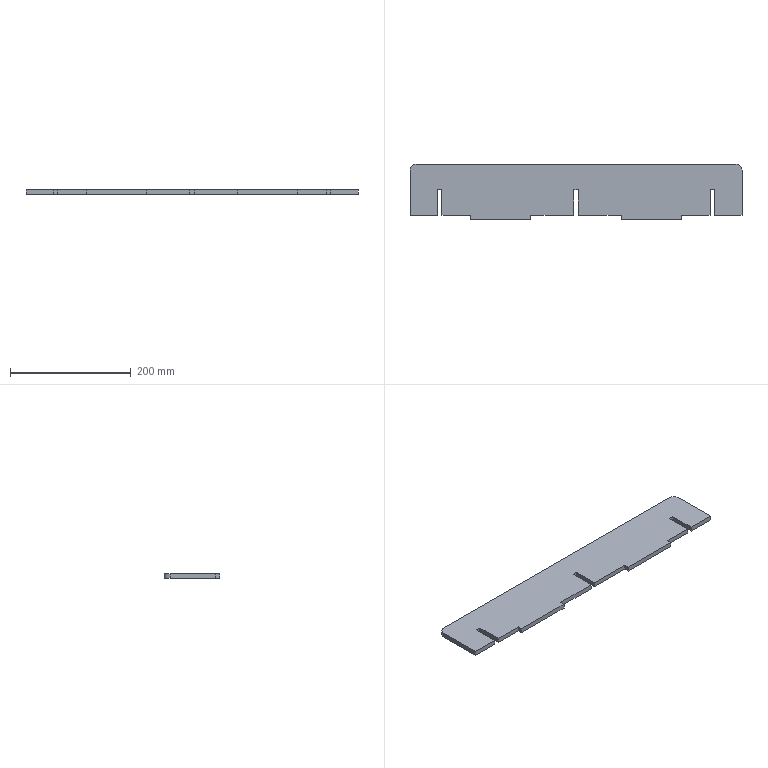Part | SolidWorks | features FlatPattern 1, SMBaseFlange 1, SheetMetal 1 | 1 solid | 28 faces | box 550 x 92.5 x 8 mm | volume 377497 mm3 | plane 26 | cylinder 2 | commonest cylinder face diameters 20 x2
STEP:
#1=CARTESIAN_POINT('',(-156.899,-982.506,0.));
#2=VERTEX_POINT('',#1);
#3=CARTESIAN_POINT('',(-111.899,-982.506,0.));
#4=VERTEX_POINT('',#3);
#5=CARTESIAN_POINT('',(-111.899,-982.506,0.));
#6=DIRECTION('',(1.,0.,0.));
#7=VECTOR('',#6,1000.);
#8=LINE('',#5,#7);
#9=EDGE_CURVE('',#2,#4,#8,.T.);
#10=ORIENTED_EDGE('',*,*,#9,.F.);
#11=CARTESIAN_POINT('',(-156.899,-982.506,-8.));
#12=VERTEX_POINT('',#11);
#13=CARTESIAN_POINT('',(-156.899,-982.506,-8.));
#14=DIRECTION('',(0.,0.,1.));
#15=VECTOR('',#14,1000.);
#16=LINE('',#13,#15);
#17=EDGE_CURVE('',#12,#2,#16,.T.);
#18=ORIENTED_EDGE('',*,*,#17,.F.);
#19=CARTESIAN_POINT('',(-111.899,-982.506,-8.));
#20=VERTEX_POINT('',#19);
#21=CARTESIAN_POINT('',(-111.899,-982.506,-8.));
#22=DIRECTION('',(1.,0.,0.));
#23=VECTOR('',#22,1000.);
#24=LINE('',#21,#23);
#25=EDGE_CURVE('',#12,#20,#24,.T.);
#26=ORIENTED_EDGE('',*,*,#25,.T.);
#27=CARTESIAN_POINT('',(-111.899,-982.506,-8.));
#28=DIRECTION('',(0.,0.,1.));
#29=VECTOR('',#28,1000.);
#30=LINE('',#27,#29);
#31=EDGE_CURVE('',#20,#4,#30,.T.);
#32=ORIENTED_EDGE('',*,*,#31,.T.);
#33=EDGE_LOOP('',(#10,#18,#26,#32));
#34=FACE_OUTER_BOUND('',#33,.T.);
#35=CARTESIAN_POINT('',(-111.899,-982.506,-8.));
#36=DIRECTION('',(0.,-1.,0.));
#37=DIRECTION('',(0.,0.,-1.));
#38=AXIS2_PLACEMENT_3D('',#35,#36,#37);
#39=PLANE('',#38);
#40=ADVANCED_FACE('',(#34),#39,.T.);
#41=CARTESIAN_POINT('',(-156.899,-907.506,0.));
#42=VERTEX_POINT('',#41);
#43=CARTESIAN_POINT('',(-156.899,-982.506,0.));
#44=DIRECTION('',(0.,-1.,0.));
#45=VECTOR('',#44,1000.);
#46=LINE('',#43,#45);
#47=EDGE_CURVE('',#42,#2,#46,.T.);
#48=ORIENTED_EDGE('',*,*,#47,.F.);
#49=CARTESIAN_POINT('',(-156.899,-907.506,-8.));
#50=VERTEX_POINT('',#49);
#51=CARTESIAN_POINT('',(-156.899,-907.506,-8.));
#52=DIRECTION('',(0.,0.,1.));
#53=VECTOR('',#52,1000.);
#54=LINE('',#51,#53);
#55=EDGE_CURVE('',#50,#42,#54,.T.);
#56=ORIENTED_EDGE('',*,*,#55,.F.);
#57=CARTESIAN_POINT('',(-156.899,-982.506,-8.));
#58=DIRECTION('',(0.,-1.,0.));
#59=VECTOR('',#58,1000.);
#60=LINE('',#57,#59);
#61=EDGE_CURVE('',#50,#12,#60,.T.);
#62=ORIENTED_EDGE('',*,*,#61,.T.);
#63=ORIENTED_EDGE('',*,*,#17,.T.);
#64=EDGE_LOOP('',(#48,#56,#62,#63));
#65=FACE_OUTER_BOUND('',#64,.T.);
#66=CARTESIAN_POINT('',(-156.899,-982.506,-8.));
#67=DIRECTION('',(-1.,0.,0.));
#68=DIRECTION('',(0.,0.,1.));
#69=AXIS2_PLACEMENT_3D('',#66,#67,#68);
#70=PLANE('',#69);
#71=ADVANCED_FACE('',(#65),#70,.T.);
#72=CARTESIAN_POINT('',(-146.899,-897.506,0.));
#73=VERTEX_POINT('',#72);
#74=CARTESIAN_POINT('',(-146.899,-907.506,0.));
#75=DIRECTION('',(0.,0.,1.));
#76=DIRECTION('',(-1.,0.,0.));
#77=AXIS2_PLACEMENT_3D('',#74,#75,#76);
#78=CIRCLE('',#77,10.);
#79=EDGE_CURVE('',#73,#42,#78,.T.);
#80=ORIENTED_EDGE('',*,*,#79,.F.);
#81=CARTESIAN_POINT('',(-146.899,-897.506,-8.));
#82=VERTEX_POINT('',#81);
#83=CARTESIAN_POINT('',(-146.899,-897.506,-8.));
#84=DIRECTION('',(0.,0.,1.));
#85=VECTOR('',#84,1000.);
#86=LINE('',#83,#85);
#87=EDGE_CURVE('',#82,#73,#86,.T.);
#88=ORIENTED_EDGE('',*,*,#87,.F.);
#89=CARTESIAN_POINT('',(-146.899,-907.506,-8.));
#90=DIRECTION('',(0.,0.,1.));
#91=DIRECTION('',(-1.,0.,0.));
#92=AXIS2_PLACEMENT_3D('',#89,#90,#91);
#93=CIRCLE('',#92,10.);
#94=EDGE_CURVE('',#82,#50,#93,.T.);
#95=ORIENTED_EDGE('',*,*,#94,.T.);
#96=ORIENTED_EDGE('',*,*,#55,.T.);
#97=EDGE_LOOP('',(#80,#88,#95,#96));
#98=FACE_OUTER_BOUND('',#97,.T.);
#99=CARTESIAN_POINT('',(-146.899,-907.506,-8.));
#100=DIRECTION('',(0.,0.,1.));
#101=DIRECTION('',(1.,0.,0.));
#102=AXIS2_PLACEMENT_3D('',#99,#100,#101);
#103=CYLINDRICAL_SURFACE('',#102,10.);
#104=ADVANCED_FACE('',(#98),#103,.T.);
#105=CARTESIAN_POINT('',(383.101,-897.506,0.));
#106=VERTEX_POINT('',#105);
#107=CARTESIAN_POINT('',(-146.899,-897.506,0.));
#108=DIRECTION('',(-1.,0.,0.));
#109=VECTOR('',#108,1000.);
#110=LINE('',#107,#109);
#111=EDGE_CURVE('',#106,#73,#110,.T.);
#112=ORIENTED_EDGE('',*,*,#111,.F.);
#113=CARTESIAN_POINT('',(383.101,-897.506,-8.));
#114=VERTEX_POINT('',#113);
#115=CARTESIAN_POINT('',(383.101,-897.506,-8.));
#116=DIRECTION('',(0.,0.,1.));
#117=VECTOR('',#116,1000.);
#118=LINE('',#115,#117);
#119=EDGE_CURVE('',#114,#106,#118,.T.);
#120=ORIENTED_EDGE('',*,*,#119,.F.);
#121=CARTESIAN_POINT('',(-146.899,-897.506,-8.));
#122=DIRECTION('',(-1.,0.,0.));
#123=VECTOR('',#122,1000.);
#124=LINE('',#121,#123);
#125=EDGE_CURVE('',#114,#82,#124,.T.);
#126=ORIENTED_EDGE('',*,*,#125,.T.);
#127=ORIENTED_EDGE('',*,*,#87,.T.);
#128=EDGE_LOOP('',(#112,#120,#126,#127));
#129=FACE_OUTER_BOUND('',#128,.T.);
#130=CARTESIAN_POINT('',(-146.899,-897.506,-8.));
#131=DIRECTION('',(0.,1.,0.));
#132=DIRECTION('',(0.,0.,1.));
#133=AXIS2_PLACEMENT_3D('',#130,#131,#132);
#134=PLANE('',#133);
#135=ADVANCED_FACE('',(#129),#134,.T.);
#136=CARTESIAN_POINT('',(393.101,-907.506,0.));
#137=VERTEX_POINT('',#136);
#138=CARTESIAN_POINT('',(383.101,-907.506,0.));
#139=DIRECTION('',(0.,0.,1.));
#140=DIRECTION('',(-1.,0.,0.));
#141=AXIS2_PLACEMENT_3D('',#138,#139,#140);
#142=CIRCLE('',#141,10.);
#143=EDGE_CURVE('',#137,#106,#142,.T.);
#144=ORIENTED_EDGE('',*,*,#143,.F.);
#145=CARTESIAN_POINT('',(393.101,-907.506,-8.));
#146=VERTEX_POINT('',#145);
#147=CARTESIAN_POINT('',(393.101,-907.506,-8.));
#148=DIRECTION('',(0.,0.,1.));
#149=VECTOR('',#148,1000.);
#150=LINE('',#147,#149);
#151=EDGE_CURVE('',#146,#137,#150,.T.);
#152=ORIENTED_EDGE('',*,*,#151,.F.);
#153=CARTESIAN_POINT('',(383.101,-907.506,-8.));
#154=DIRECTION('',(0.,0.,1.));
#155=DIRECTION('',(-1.,0.,0.));
#156=AXIS2_PLACEMENT_3D('',#153,#154,#155);
#157=CIRCLE('',#156,10.);
#158=EDGE_CURVE('',#146,#114,#157,.T.);
#159=ORIENTED_EDGE('',*,*,#158,.T.);
#160=ORIENTED_EDGE('',*,*,#119,.T.);
#161=EDGE_LOOP('',(#144,#152,#159,#160));
#162=FACE_OUTER_BOUND('',#161,.T.);
#163=CARTESIAN_POINT('',(383.101,-907.506,-8.));
#164=DIRECTION('',(0.,0.,1.));
#165=DIRECTION('',(1.,0.,0.));
#166=AXIS2_PLACEMENT_3D('',#163,#164,#165);
#167=CYLINDRICAL_SURFACE('',#166,10.);
#168=ADVANCED_FACE('',(#162),#167,.T.);
#169=CARTESIAN_POINT('',(393.101,-982.506,0.));
#170=VERTEX_POINT('',#169);
#171=CARTESIAN_POINT('',(393.101,-907.506,0.));
#172=DIRECTION('',(0.,1.,0.));
#173=VECTOR('',#172,1000.);
#174=LINE('',#171,#173);
#175=EDGE_CURVE('',#170,#137,#174,.T.);
#176=ORIENTED_EDGE('',*,*,#175,.F.);
#177=CARTESIAN_POINT('',(393.101,-982.506,-8.));
#178=VERTEX_POINT('',#177);
#179=CARTESIAN_POINT('',(393.101,-982.506,-8.));
#180=DIRECTION('',(0.,0.,1.));
#181=VECTOR('',#180,1000.);
#182=LINE('',#179,#181);
#183=EDGE_CURVE('',#178,#170,#182,.T.);
#184=ORIENTED_EDGE('',*,*,#183,.F.);
#185=CARTESIAN_POINT('',(393.101,-907.506,-8.));
#186=DIRECTION('',(0.,1.,0.));
#187=VECTOR('',#186,1000.);
#188=LINE('',#185,#187);
#189=EDGE_CURVE('',#178,#146,#188,.T.);
#190=ORIENTED_EDGE('',*,*,#189,.T.);
#191=ORIENTED_EDGE('',*,*,#151,.T.);
#192=EDGE_LOOP('',(#176,#184,#190,#191));
#193=FACE_OUTER_BOUND('',#192,.T.);
#194=CARTESIAN_POINT('',(393.101,-907.506,-8.));
#195=DIRECTION('',(1.,0.,0.));
#196=DIRECTION('',(0.,0.,-1.));
#197=AXIS2_PLACEMENT_3D('',#194,#195,#196);
#198=PLANE('',#197);
#199=ADVANCED_FACE('',(#193),#198,.T.);
#200=CARTESIAN_POINT('',(348.101,-982.506,0.));
#201=VERTEX_POINT('',#200);
#202=CARTESIAN_POINT('',(393.101,-982.506,0.));
#203=DIRECTION('',(1.,0.,0.));
#204=VECTOR('',#203,1000.);
#205=LINE('',#202,#204);
#206=EDGE_CURVE('',#201,#170,#205,.T.);
#207=ORIENTED_EDGE('',*,*,#206,.F.);
#208=CARTESIAN_POINT('',(348.101,-982.506,-8.));
#209=VERTEX_POINT('',#208);
#210=CARTESIAN_POINT('',(348.101,-982.506,-8.));
#211=DIRECTION('',(0.,0.,1.));
#212=VECTOR('',#211,1000.);
#213=LINE('',#210,#212);
#214=EDGE_CURVE('',#209,#201,#213,.T.);
#215=ORIENTED_EDGE('',*,*,#214,.F.);
#216=CARTESIAN_POINT('',(393.101,-982.506,-8.));
#217=DIRECTION('',(1.,0.,0.));
#218=VECTOR('',#217,1000.);
#219=LINE('',#216,#218);
#220=EDGE_CURVE('',#209,#178,#219,.T.);
#221=ORIENTED_EDGE('',*,*,#220,.T.);
#222=ORIENTED_EDGE('',*,*,#183,.T.);
#223=EDGE_LOOP('',(#207,#215,#221,#222));
#224=FACE_OUTER_BOUND('',#223,.T.);
#225=CARTESIAN_POINT('',(393.101,-982.506,-8.));
#226=DIRECTION('',(0.,-1.,0.));
#227=DIRECTION('',(0.,0.,-1.));
#228=AXIS2_PLACEMENT_3D('',#225,#226,#227);
#229=PLANE('',#228);
#230=ADVANCED_FACE('',(#224),#229,.T.);
#231=CARTESIAN_POINT('',(348.101,-940.006,0.));
#232=VERTEX_POINT('',#231);
#233=CARTESIAN_POINT('',(348.101,-982.506,0.));
#234=DIRECTION('',(0.,-1.,0.));
#235=VECTOR('',#234,1000.);
#236=LINE('',#233,#235);
#237=EDGE_CURVE('',#232,#201,#236,.T.);
#238=ORIENTED_EDGE('',*,*,#237,.F.);
#239=CARTESIAN_POINT('',(348.101,-940.006,-8.));
#240=VERTEX_POINT('',#239);
#241=CARTESIAN_POINT('',(348.101,-940.006,-8.));
#242=DIRECTION('',(0.,0.,1.));
#243=VECTOR('',#242,1000.);
#244=LINE('',#241,#243);
#245=EDGE_CURVE('',#240,#232,#244,.T.);
#246=ORIENTED_EDGE('',*,*,#245,.F.);
#247=CARTESIAN_POINT('',(348.101,-982.506,-8.));
#248=DIRECTION('',(0.,-1.,0.));
#249=VECTOR('',#248,1000.);
#250=LINE('',#247,#249);
#251=EDGE_CURVE('',#240,#209,#250,.T.);
#252=ORIENTED_EDGE('',*,*,#251,.T.);
#253=ORIENTED_EDGE('',*,*,#214,.T.);
#254=EDGE_LOOP('',(#238,#246,#252,#253));
#255=FACE_OUTER_BOUND('',#254,.T.);
#256=CARTESIAN_POINT('',(348.101,-982.506,-8.));
#257=DIRECTION('',(-1.,0.,0.));
#258=DIRECTION('',(0.,0.,1.));
#259=AXIS2_PLACEMENT_3D('',#256,#257,#258);
#260=PLANE('',#259);
#261=ADVANCED_FACE('',(#255),#260,.T.);
#262=CARTESIAN_POINT('',(340.101,-940.006,0.));
#263=VERTEX_POINT('',#262);
#264=CARTESIAN_POINT('',(348.101,-940.006,0.));
#265=DIRECTION('',(1.,0.,0.));
#266=VECTOR('',#265,1000.);
#267=LINE('',#264,#266);
#268=EDGE_CURVE('',#263,#232,#267,.T.);
#269=ORIENTED_EDGE('',*,*,#268,.F.);
#270=CARTESIAN_POINT('',(340.101,-940.006,-8.));
#271=VERTEX_POINT('',#270);
#272=CARTESIAN_POINT('',(340.101,-940.006,-8.));
#273=DIRECTION('',(0.,0.,1.));
#274=VECTOR('',#273,1000.);
#275=LINE('',#272,#274);
#276=EDGE_CURVE('',#271,#263,#275,.T.);
#277=ORIENTED_EDGE('',*,*,#276,.F.);
#278=CARTESIAN_POINT('',(348.101,-940.006,-8.));
#279=DIRECTION('',(1.,0.,0.));
#280=VECTOR('',#279,1000.);
#281=LINE('',#278,#280);
#282=EDGE_CURVE('',#271,#240,#281,.T.);
#283=ORIENTED_EDGE('',*,*,#282,.T.);
#284=ORIENTED_EDGE('',*,*,#245,.T.);
#285=EDGE_LOOP('',(#269,#277,#283,#284));
#286=FACE_OUTER_BOUND('',#285,.T.);
#287=CARTESIAN_POINT('',(348.101,-940.006,-8.));
#288=DIRECTION('',(0.,-1.,0.));
#289=DIRECTION('',(0.,0.,-1.));
#290=AXIS2_PLACEMENT_3D('',#287,#288,#289);
#291=PLANE('',#290);
#292=ADVANCED_FACE('',(#286),#291,.T.);
#293=CARTESIAN_POINT('',(340.101,-982.506,0.));
#294=VERTEX_POINT('',#293);
#295=CARTESIAN_POINT('',(340.101,-940.006,0.));
#296=DIRECTION('',(0.,1.,0.));
#297=VECTOR('',#296,1000.);
#298=LINE('',#295,#297);
#299=EDGE_CURVE('',#294,#263,#298,.T.);
#300=ORIENTED_EDGE('',*,*,#299,.F.);
#301=CARTESIAN_POINT('',(340.101,-982.506,-8.));
#302=VERTEX_POINT('',#301);
#303=CARTESIAN_POINT('',(340.101,-982.506,-8.));
#304=DIRECTION('',(0.,0.,1.));
#305=VECTOR('',#304,1000.);
#306=LINE('',#303,#305);
#307=EDGE_CURVE('',#302,#294,#306,.T.);
#308=ORIENTED_EDGE('',*,*,#307,.F.);
#309=CARTESIAN_POINT('',(340.101,-940.006,-8.));
#310=DIRECTION('',(0.,1.,0.));
#311=VECTOR('',#310,1000.);
#312=LINE('',#309,#311);
#313=EDGE_CURVE('',#302,#271,#312,.T.);
#314=ORIENTED_EDGE('',*,*,#313,.T.);
#315=ORIENTED_EDGE('',*,*,#276,.T.);
#316=EDGE_LOOP('',(#300,#308,#314,#315));
#317=FACE_OUTER_BOUND('',#316,.T.);
#318=CARTESIAN_POINT('',(340.101,-940.006,-8.));
#319=DIRECTION('',(1.,0.,0.));
#320=DIRECTION('',(0.,0.,-1.));
#321=AXIS2_PLACEMENT_3D('',#318,#319,#320);
#322=PLANE('',#321);
#323=ADVANCED_FACE('',(#317),#322,.T.);
#324=CARTESIAN_POINT('',(293.101,-982.506,0.));
#325=VERTEX_POINT('',#324);
#326=CARTESIAN_POINT('',(340.101,-982.506,0.));
#327=DIRECTION('',(1.,0.,0.));
#328=VECTOR('',#327,1000.);
#329=LINE('',#326,#328);
#330=EDGE_CURVE('',#325,#294,#329,.T.);
#331=ORIENTED_EDGE('',*,*,#330,.F.);
#332=CARTESIAN_POINT('',(293.101,-982.506,-8.));
#333=VERTEX_POINT('',#332);
#334=CARTESIAN_POINT('',(293.101,-982.506,-8.));
#335=DIRECTION('',(0.,0.,1.));
#336=VECTOR('',#335,1000.);
#337=LINE('',#334,#336);
#338=EDGE_CURVE('',#333,#325,#337,.T.);
#339=ORIENTED_EDGE('',*,*,#338,.F.);
#340=CARTESIAN_POINT('',(340.101,-982.506,-8.));
#341=DIRECTION('',(1.,0.,0.));
#342=VECTOR('',#341,1000.);
#343=LINE('',#340,#342);
#344=EDGE_CURVE('',#333,#302,#343,.T.);
#345=ORIENTED_EDGE('',*,*,#344,.T.);
#346=ORIENTED_EDGE('',*,*,#307,.T.);
#347=EDGE_LOOP('',(#331,#339,#345,#346));
#348=FACE_OUTER_BOUND('',#347,.T.);
#349=CARTESIAN_POINT('',(340.101,-982.506,-8.));
#350=DIRECTION('',(0.,-1.,0.));
#351=DIRECTION('',(1.,0.,0.));
#352=AXIS2_PLACEMENT_3D('',#349,#350,#351);
#353=PLANE('',#352);
#354=ADVANCED_FACE('',(#348),#353,.T.);
#355=CARTESIAN_POINT('',(293.101,-990.006,0.));
#356=VERTEX_POINT('',#355);
#357=CARTESIAN_POINT('',(293.101,-990.006,0.));
#358=DIRECTION('',(0.,1.,0.));
#359=VECTOR('',#358,1000.);
#360=LINE('',#357,#359);
#361=EDGE_CURVE('',#356,#325,#360,.T.);
#362=ORIENTED_EDGE('',*,*,#361,.F.);
#363=CARTESIAN_POINT('',(293.101,-990.006,-8.));
#364=VERTEX_POINT('',#363);
#365=CARTESIAN_POINT('',(293.101,-990.006,-8.));
#366=DIRECTION('',(0.,0.,1.));
#367=VECTOR('',#366,1000.);
#368=LINE('',#365,#367);
#369=EDGE_CURVE('',#364,#356,#368,.T.);
#370=ORIENTED_EDGE('',*,*,#369,.F.);
#371=CARTESIAN_POINT('',(293.101,-990.006,-8.));
#372=DIRECTION('',(0.,1.,0.));
#373=VECTOR('',#372,1000.);
#374=LINE('',#371,#373);
#375=EDGE_CURVE('',#364,#333,#374,.T.);
#376=ORIENTED_EDGE('',*,*,#375,.T.);
#377=ORIENTED_EDGE('',*,*,#338,.T.);
#378=EDGE_LOOP('',(#362,#370,#376,#377));
#379=FACE_OUTER_BOUND('',#378,.T.);
#380=CARTESIAN_POINT('',(293.101,-990.006,-8.));
#381=DIRECTION('',(1.,0.,0.));
#382=DIRECTION('',(0.,0.,-1.));
#383=AXIS2_PLACEMENT_3D('',#380,#381,#382);
#384=PLANE('',#383);
#385=ADVANCED_FACE('',(#379),#384,.T.);
#386=CARTESIAN_POINT('',(193.101,-990.006,0.));
#387=VERTEX_POINT('',#386);
#388=CARTESIAN_POINT('',(193.101,-990.006,0.));
#389=DIRECTION('',(1.,0.,0.));
#390=VECTOR('',#389,1000.);
#391=LINE('',#388,#390);
#392=EDGE_CURVE('',#387,#356,#391,.T.);
#393=ORIENTED_EDGE('',*,*,#392,.F.);
#394=CARTESIAN_POINT('',(193.101,-990.006,-8.));
#395=VERTEX_POINT('',#394);
#396=CARTESIAN_POINT('',(193.101,-990.006,-8.));
#397=DIRECTION('',(0.,0.,1.));
#398=VECTOR('',#397,1000.);
#399=LINE('',#396,#398);
#400=EDGE_CURVE('',#395,#387,#399,.T.);
#401=ORIENTED_EDGE('',*,*,#400,.F.);
#402=CARTESIAN_POINT('',(193.101,-990.006,-8.));
#403=DIRECTION('',(1.,0.,0.));
#404=VECTOR('',#403,1000.);
#405=LINE('',#402,#404);
#406=EDGE_CURVE('',#395,#364,#405,.T.);
#407=ORIENTED_EDGE('',*,*,#406,.T.);
#408=ORIENTED_EDGE('',*,*,#369,.T.);
#409=EDGE_LOOP('',(#393,#401,#407,#408));
#410=FACE_OUTER_BOUND('',#409,.T.);
#411=CARTESIAN_POINT('',(193.101,-990.006,-8.));
#412=DIRECTION('',(0.,-1.,0.));
#413=DIRECTION('',(0.,0.,-1.));
#414=AXIS2_PLACEMENT_3D('',#411,#412,#413);
#415=PLANE('',#414);
#416=ADVANCED_FACE('',(#410),#415,.T.);
#417=CARTESIAN_POINT('',(193.101,-982.506,0.));
#418=VERTEX_POINT('',#417);
#419=CARTESIAN_POINT('',(193.101,-982.506,0.));
#420=DIRECTION('',(0.,-1.,0.));
#421=VECTOR('',#420,1000.);
#422=LINE('',#419,#421);
#423=EDGE_CURVE('',#418,#387,#422,.T.);
#424=ORIENTED_EDGE('',*,*,#423,.F.);
#425=CARTESIAN_POINT('',(193.101,-982.506,-8.));
#426=VERTEX_POINT('',#425);
#427=CARTESIAN_POINT('',(193.101,-982.506,-8.));
#428=DIRECTION('',(0.,0.,1.));
#429=VECTOR('',#428,1000.);
#430=LINE('',#427,#429);
#431=EDGE_CURVE('',#426,#418,#430,.T.);
#432=ORIENTED_EDGE('',*,*,#431,.F.);
#433=CARTESIAN_POINT('',(193.101,-982.506,-8.));
#434=DIRECTION('',(0.,-1.,0.));
#435=VECTOR('',#434,1000.);
#436=LINE('',#433,#435);
#437=EDGE_CURVE('',#426,#395,#436,.T.);
#438=ORIENTED_EDGE('',*,*,#437,.T.);
#439=ORIENTED_EDGE('',*,*,#400,.T.);
#440=EDGE_LOOP('',(#424,#432,#438,#439));
#441=FACE_OUTER_BOUND('',#440,.T.);
#442=CARTESIAN_POINT('',(193.101,-982.506,-8.));
#443=DIRECTION('',(-1.,0.,0.));
#444=DIRECTION('',(0.,0.,1.));
#445=AXIS2_PLACEMENT_3D('',#442,#443,#444);
#446=PLANE('',#445);
#447=ADVANCED_FACE('',(#441),#446,.T.);
#448=CARTESIAN_POINT('',(122.101,-982.506,0.));
#449=VERTEX_POINT('',#448);
#450=CARTESIAN_POINT('',(193.101,-982.506,0.));
#451=DIRECTION('',(1.,0.,0.));
#452=VECTOR('',#451,1000.);
#453=LINE('',#450,#452);
#454=EDGE_CURVE('',#449,#418,#453,.T.);
#455=ORIENTED_EDGE('',*,*,#454,.F.);
#456=CARTESIAN_POINT('',(122.101,-982.506,-8.));
#457=VERTEX_POINT('',#456);
#458=CARTESIAN_POINT('',(122.101,-982.506,-8.));
#459=DIRECTION('',(0.,0.,1.));
#460=VECTOR('',#459,1000.);
#461=LINE('',#458,#460);
#462=EDGE_CURVE('',#457,#449,#461,.T.);
#463=ORIENTED_EDGE('',*,*,#462,.F.);
#464=CARTESIAN_POINT('',(193.101,-982.506,-8.));
#465=DIRECTION('',(1.,0.,0.));
#466=VECTOR('',#465,1000.);
#467=LINE('',#464,#466);
#468=EDGE_CURVE('',#457,#426,#467,.T.);
#469=ORIENTED_EDGE('',*,*,#468,.T.);
#470=ORIENTED_EDGE('',*,*,#431,.T.);
#471=EDGE_LOOP('',(#455,#463,#469,#470));
#472=FACE_OUTER_BOUND('',#471,.T.);
#473=CARTESIAN_POINT('',(193.101,-982.506,-8.));
#474=DIRECTION('',(0.,-1.,0.));
#475=DIRECTION('',(1.,0.,0.));
#476=AXIS2_PLACEMENT_3D('',#473,#474,#475);
#477=PLANE('',#476);
#478=ADVANCED_FACE('',(#472),#477,.T.);
#479=CARTESIAN_POINT('',(122.101,-940.006,0.));
#480=VERTEX_POINT('',#479);
#481=CARTESIAN_POINT('',(122.101,-982.506,0.));
#482=DIRECTION('',(0.,-1.,0.));
#483=VECTOR('',#482,1000.);
#484=LINE('',#481,#483);
#485=EDGE_CURVE('',#480,#449,#484,.T.);
#486=ORIENTED_EDGE('',*,*,#485,.F.);
#487=CARTESIAN_POINT('',(122.101,-940.006,-8.));
#488=VERTEX_POINT('',#487);
#489=CARTESIAN_POINT('',(122.101,-940.006,-8.));
#490=DIRECTION('',(0.,0.,1.));
#491=VECTOR('',#490,1000.);
#492=LINE('',#489,#491);
#493=EDGE_CURVE('',#488,#480,#492,.T.);
#494=ORIENTED_EDGE('',*,*,#493,.F.);
#495=CARTESIAN_POINT('',(122.101,-982.506,-8.));
#496=DIRECTION('',(0.,-1.,0.));
#497=VECTOR('',#496,1000.);
#498=LINE('',#495,#497);
#499=EDGE_CURVE('',#488,#457,#498,.T.);
#500=ORIENTED_EDGE('',*,*,#499,.T.);
#501=ORIENTED_EDGE('',*,*,#462,.T.);
#502=EDGE_LOOP('',(#486,#494,#500,#501));
#503=FACE_OUTER_BOUND('',#502,.T.);
#504=CARTESIAN_POINT('',(122.101,-982.506,-8.));
#505=DIRECTION('',(-1.,0.,0.));
#506=DIRECTION('',(0.,0.,1.));
#507=AXIS2_PLACEMENT_3D('',#504,#505,#506);
#508=PLANE('',#507);
#509=ADVANCED_FACE('',(#503),#508,.T.);
#510=CARTESIAN_POINT('',(114.101,-940.006,0.));
#511=VERTEX_POINT('',#510);
#512=CARTESIAN_POINT('',(122.101,-940.006,0.));
#513=DIRECTION('',(1.,0.,0.));
#514=VECTOR('',#513,1000.);
#515=LINE('',#512,#514);
#516=EDGE_CURVE('',#511,#480,#515,.T.);
#517=ORIENTED_EDGE('',*,*,#516,.F.);
#518=CARTESIAN_POINT('',(114.101,-940.006,-8.));
#519=VERTEX_POINT('',#518);
#520=CARTESIAN_POINT('',(114.101,-940.006,-8.));
#521=DIRECTION('',(0.,0.,1.));
#522=VECTOR('',#521,1000.);
#523=LINE('',#520,#522);
#524=EDGE_CURVE('',#519,#511,#523,.T.);
#525=ORIENTED_EDGE('',*,*,#524,.F.);
#526=CARTESIAN_POINT('',(122.101,-940.006,-8.));
#527=DIRECTION('',(1.,0.,0.));
#528=VECTOR('',#527,1000.);
#529=LINE('',#526,#528);
#530=EDGE_CURVE('',#519,#488,#529,.T.);
#531=ORIENTED_EDGE('',*,*,#530,.T.);
#532=ORIENTED_EDGE('',*,*,#493,.T.);
#533=EDGE_LOOP('',(#517,#525,#531,#532));
#534=FACE_OUTER_BOUND('',#533,.T.);
#535=CARTESIAN_POINT('',(122.101,-940.006,-8.));
#536=DIRECTION('',(0.,-1.,0.));
#537=DIRECTION('',(0.,0.,-1.));
#538=AXIS2_PLACEMENT_3D('',#535,#536,#537);
#539=PLANE('',#538);
#540=ADVANCED_FACE('',(#534),#539,.T.);
#541=CARTESIAN_POINT('',(114.101,-982.506,0.));
#542=VERTEX_POINT('',#541);
#543=CARTESIAN_POINT('',(114.101,-940.006,0.));
#544=DIRECTION('',(0.,1.,0.));
#545=VECTOR('',#544,1000.);
#546=LINE('',#543,#545);
#547=EDGE_CURVE('',#542,#511,#546,.T.);
#548=ORIENTED_EDGE('',*,*,#547,.F.);
#549=CARTESIAN_POINT('',(114.101,-982.506,-8.));
#550=VERTEX_POINT('',#549);
#551=CARTESIAN_POINT('',(114.101,-982.506,-8.));
#552=DIRECTION('',(0.,0.,1.));
#553=VECTOR('',#552,1000.);
#554=LINE('',#551,#553);
#555=EDGE_CURVE('',#550,#542,#554,.T.);
#556=ORIENTED_EDGE('',*,*,#555,.F.);
#557=CARTESIAN_POINT('',(114.101,-940.006,-8.));
#558=DIRECTION('',(0.,1.,0.));
#559=VECTOR('',#558,1000.);
#560=LINE('',#557,#559);
#561=EDGE_CURVE('',#550,#519,#560,.T.);
#562=ORIENTED_EDGE('',*,*,#561,.T.);
#563=ORIENTED_EDGE('',*,*,#524,.T.);
#564=EDGE_LOOP('',(#548,#556,#562,#563));
#565=FACE_OUTER_BOUND('',#564,.T.);
#566=CARTESIAN_POINT('',(114.101,-940.006,-8.));
#567=DIRECTION('',(1.,0.,0.));
#568=DIRECTION('',(0.,0.,-1.));
#569=AXIS2_PLACEMENT_3D('',#566,#567,#568);
#570=PLANE('',#569);
#571=ADVANCED_FACE('',(#565),#570,.T.);
#572=CARTESIAN_POINT('',(43.101,-982.506,0.));
#573=VERTEX_POINT('',#572);
#574=CARTESIAN_POINT('',(114.101,-982.506,0.));
#575=DIRECTION('',(1.,0.,0.));
#576=VECTOR('',#575,1000.);
#577=LINE('',#574,#576);
#578=EDGE_CURVE('',#573,#542,#577,.T.);
#579=ORIENTED_EDGE('',*,*,#578,.F.);
#580=CARTESIAN_POINT('',(43.101,-982.506,-8.));
#581=VERTEX_POINT('',#580);
#582=CARTESIAN_POINT('',(43.101,-982.506,-8.));
#583=DIRECTION('',(0.,0.,1.));
#584=VECTOR('',#583,1000.);
#585=LINE('',#582,#584);
#586=EDGE_CURVE('',#581,#573,#585,.T.);
#587=ORIENTED_EDGE('',*,*,#586,.F.);
#588=CARTESIAN_POINT('',(114.101,-982.506,-8.));
#589=DIRECTION('',(1.,0.,0.));
#590=VECTOR('',#589,1000.);
#591=LINE('',#588,#590);
#592=EDGE_CURVE('',#581,#550,#591,.T.);
#593=ORIENTED_EDGE('',*,*,#592,.T.);
#594=ORIENTED_EDGE('',*,*,#555,.T.);
#595=EDGE_LOOP('',(#579,#587,#593,#594));
#596=FACE_OUTER_BOUND('',#595,.T.);
#597=CARTESIAN_POINT('',(114.101,-982.506,-8.));
#598=DIRECTION('',(0.,-1.,0.));
#599=DIRECTION('',(1.,0.,0.));
#600=AXIS2_PLACEMENT_3D('',#597,#598,#599);
#601=PLANE('',#600);
#602=ADVANCED_FACE('',(#596),#601,.T.);
#603=CARTESIAN_POINT('',(43.101,-990.006,0.));
#604=VERTEX_POINT('',#603);
#605=CARTESIAN_POINT('',(43.101,-990.006,0.));
#606=DIRECTION('',(0.,1.,0.));
#607=VECTOR('',#606,1000.);
#608=LINE('',#605,#607);
#609=EDGE_CURVE('',#604,#573,#608,.T.);
#610=ORIENTED_EDGE('',*,*,#609,.F.);
#611=CARTESIAN_POINT('',(43.101,-990.006,-8.));
#612=VERTEX_POINT('',#611);
#613=CARTESIAN_POINT('',(43.101,-990.006,-8.));
#614=DIRECTION('',(0.,0.,1.));
#615=VECTOR('',#614,1000.);
#616=LINE('',#613,#615);
#617=EDGE_CURVE('',#612,#604,#616,.T.);
#618=ORIENTED_EDGE('',*,*,#617,.F.);
#619=CARTESIAN_POINT('',(43.101,-990.006,-8.));
#620=DIRECTION('',(0.,1.,0.));
#621=VECTOR('',#620,1000.);
#622=LINE('',#619,#621);
#623=EDGE_CURVE('',#612,#581,#622,.T.);
#624=ORIENTED_EDGE('',*,*,#623,.T.);
#625=ORIENTED_EDGE('',*,*,#586,.T.);
#626=EDGE_LOOP('',(#610,#618,#624,#625));
#627=FACE_OUTER_BOUND('',#626,.T.);
#628=CARTESIAN_POINT('',(43.101,-990.006,-8.));
#629=DIRECTION('',(1.,0.,0.));
#630=DIRECTION('',(0.,1.,0.));
#631=AXIS2_PLACEMENT_3D('',#628,#629,#630);
#632=PLANE('',#631);
#633=ADVANCED_FACE('',(#627),#632,.T.);
#634=CARTESIAN_POINT('',(-56.899,-990.006,0.));
#635=VERTEX_POINT('',#634);
#636=CARTESIAN_POINT('',(-56.899,-990.006,0.));
#637=DIRECTION('',(1.,0.,0.));
#638=VECTOR('',#637,1000.);
#639=LINE('',#636,#638);
#640=EDGE_CURVE('',#635,#604,#639,.T.);
#641=ORIENTED_EDGE('',*,*,#640,.F.);
#642=CARTESIAN_POINT('',(-56.899,-990.006,-8.));
#643=VERTEX_POINT('',#642);
#644=CARTESIAN_POINT('',(-56.899,-990.006,-8.));
#645=DIRECTION('',(0.,0.,1.));
#646=VECTOR('',#645,1000.);
#647=LINE('',#644,#646);
#648=EDGE_CURVE('',#643,#635,#647,.T.);
#649=ORIENTED_EDGE('',*,*,#648,.F.);
#650=CARTESIAN_POINT('',(-56.899,-990.006,-8.));
#651=DIRECTION('',(1.,0.,0.));
#652=VECTOR('',#651,1000.);
#653=LINE('',#650,#652);
#654=EDGE_CURVE('',#643,#612,#653,.T.);
#655=ORIENTED_EDGE('',*,*,#654,.T.);
#656=ORIENTED_EDGE('',*,*,#617,.T.);
#657=EDGE_LOOP('',(#641,#649,#655,#656));
#658=FACE_OUTER_BOUND('',#657,.T.);
#659=CARTESIAN_POINT('',(-56.899,-990.006,-8.));
#660=DIRECTION('',(0.,-1.,0.));
#661=DIRECTION('',(1.,0.,0.));
#662=AXIS2_PLACEMENT_3D('',#659,#660,#661);
#663=PLANE('',#662);
#664=ADVANCED_FACE('',(#658),#663,.T.);
#665=CARTESIAN_POINT('',(-56.899,-982.506,0.));
#666=VERTEX_POINT('',#665);
#667=CARTESIAN_POINT('',(-56.899,-982.506,0.));
#668=DIRECTION('',(0.,-1.,0.));
#669=VECTOR('',#668,1000.);
#670=LINE('',#667,#669);
#671=EDGE_CURVE('',#666,#635,#670,.T.);
#672=ORIENTED_EDGE('',*,*,#671,.F.);
#673=CARTESIAN_POINT('',(-56.899,-982.506,-8.));
#674=VERTEX_POINT('',#673);
#675=CARTESIAN_POINT('',(-56.899,-982.506,-8.));
#676=DIRECTION('',(0.,0.,1.));
#677=VECTOR('',#676,1000.);
#678=LINE('',#675,#677);
#679=EDGE_CURVE('',#674,#666,#678,.T.);
#680=ORIENTED_EDGE('',*,*,#679,.F.);
#681=CARTESIAN_POINT('',(-56.899,-982.506,-8.));
#682=DIRECTION('',(0.,-1.,0.));
#683=VECTOR('',#682,1000.);
#684=LINE('',#681,#683);
#685=EDGE_CURVE('',#674,#643,#684,.T.);
#686=ORIENTED_EDGE('',*,*,#685,.T.);
#687=ORIENTED_EDGE('',*,*,#648,.T.);
#688=EDGE_LOOP('',(#672,#680,#686,#687));
#689=FACE_OUTER_BOUND('',#688,.T.);
#690=CARTESIAN_POINT('',(-56.899,-982.506,-8.));
#691=DIRECTION('',(-1.,0.,0.));
#692=DIRECTION('',(0.,0.,1.));
#693=AXIS2_PLACEMENT_3D('',#690,#691,#692);
#694=PLANE('',#693);
#695=ADVANCED_FACE('',(#689),#694,.T.);
#696=CARTESIAN_POINT('',(-103.899,-982.506,0.));
#697=VERTEX_POINT('',#696);
#698=CARTESIAN_POINT('',(-56.899,-982.506,0.));
#699=DIRECTION('',(1.,0.,0.));
#700=VECTOR('',#699,1000.);
#701=LINE('',#698,#700);
#702=EDGE_CURVE('',#697,#666,#701,.T.);
#703=ORIENTED_EDGE('',*,*,#702,.F.);
#704=CARTESIAN_POINT('',(-103.899,-982.506,-8.));
#705=VERTEX_POINT('',#704);
#706=CARTESIAN_POINT('',(-103.899,-982.506,-8.));
#707=DIRECTION('',(0.,0.,1.));
#708=VECTOR('',#707,1000.);
#709=LINE('',#706,#708);
#710=EDGE_CURVE('',#705,#697,#709,.T.);
#711=ORIENTED_EDGE('',*,*,#710,.F.);
#712=CARTESIAN_POINT('',(-56.899,-982.506,-8.));
#713=DIRECTION('',(1.,0.,0.));
#714=VECTOR('',#713,1000.);
#715=LINE('',#712,#714);
#716=EDGE_CURVE('',#705,#674,#715,.T.);
#717=ORIENTED_EDGE('',*,*,#716,.T.);
#718=ORIENTED_EDGE('',*,*,#679,.T.);
#719=EDGE_LOOP('',(#703,#711,#717,#718));
#720=FACE_OUTER_BOUND('',#719,.T.);
#721=CARTESIAN_POINT('',(-56.899,-982.506,-8.));
#722=DIRECTION('',(0.,-1.,0.));
#723=DIRECTION('',(1.,0.,0.));
#724=AXIS2_PLACEMENT_3D('',#721,#722,#723);
#725=PLANE('',#724);
#726=ADVANCED_FACE('',(#720),#725,.T.);
#727=CARTESIAN_POINT('',(-103.899,-940.006,0.));
#728=VERTEX_POINT('',#727);
#729=CARTESIAN_POINT('',(-103.899,-982.506,0.));
#730=DIRECTION('',(0.,-1.,0.));
#731=VECTOR('',#730,1000.);
#732=LINE('',#729,#731);
#733=EDGE_CURVE('',#728,#697,#732,.T.);
#734=ORIENTED_EDGE('',*,*,#733,.F.);
#735=CARTESIAN_POINT('',(-103.899,-940.006,-8.));
#736=VERTEX_POINT('',#735);
#737=CARTESIAN_POINT('',(-103.899,-940.006,-8.));
#738=DIRECTION('',(0.,0.,1.));
#739=VECTOR('',#738,1000.);
#740=LINE('',#737,#739);
#741=EDGE_CURVE('',#736,#728,#740,.T.);
#742=ORIENTED_EDGE('',*,*,#741,.F.);
#743=CARTESIAN_POINT('',(-103.899,-982.506,-8.));
#744=DIRECTION('',(0.,-1.,0.));
#745=VECTOR('',#744,1000.);
#746=LINE('',#743,#745);
#747=EDGE_CURVE('',#736,#705,#746,.T.);
#748=ORIENTED_EDGE('',*,*,#747,.T.);
#749=ORIENTED_EDGE('',*,*,#710,.T.);
#750=EDGE_LOOP('',(#734,#742,#748,#749));
#751=FACE_OUTER_BOUND('',#750,.T.);
#752=CARTESIAN_POINT('',(-103.899,-982.506,-8.));
#753=DIRECTION('',(-1.,0.,0.));
#754=DIRECTION('',(0.,0.,1.));
#755=AXIS2_PLACEMENT_3D('',#752,#753,#754);
#756=PLANE('',#755);
#757=ADVANCED_FACE('',(#751),#756,.T.);
#758=CARTESIAN_POINT('',(-111.899,-940.006,0.));
#759=VERTEX_POINT('',#758);
#760=CARTESIAN_POINT('',(-103.899,-940.006,0.));
#761=DIRECTION('',(1.,0.,0.));
#762=VECTOR('',#761,1000.);
#763=LINE('',#760,#762);
#764=EDGE_CURVE('',#759,#728,#763,.T.);
#765=ORIENTED_EDGE('',*,*,#764,.F.);
#766=CARTESIAN_POINT('',(-111.899,-940.006,-8.));
#767=VERTEX_POINT('',#766);
#768=CARTESIAN_POINT('',(-111.899,-940.006,-8.));
#769=DIRECTION('',(0.,0.,1.));
#770=VECTOR('',#769,1000.);
#771=LINE('',#768,#770);
#772=EDGE_CURVE('',#767,#759,#771,.T.);
#773=ORIENTED_EDGE('',*,*,#772,.F.);
#774=CARTESIAN_POINT('',(-103.899,-940.006,-8.));
#775=DIRECTION('',(1.,0.,0.));
#776=VECTOR('',#775,1000.);
#777=LINE('',#774,#776);
#778=EDGE_CURVE('',#767,#736,#777,.T.);
#779=ORIENTED_EDGE('',*,*,#778,.T.);
#780=ORIENTED_EDGE('',*,*,#741,.T.);
#781=EDGE_LOOP('',(#765,#773,#779,#780));
#782=FACE_OUTER_BOUND('',#781,.T.);
#783=CARTESIAN_POINT('',(-103.899,-940.006,-8.));
#784=DIRECTION('',(0.,-1.,0.));
#785=DIRECTION('',(0.,0.,-1.));
#786=AXIS2_PLACEMENT_3D('',#783,#784,#785);
#787=PLANE('',#786);
#788=ADVANCED_FACE('',(#782),#787,.T.);
#789=CARTESIAN_POINT('',(-111.899,-940.006,0.));
#790=DIRECTION('',(0.,1.,0.));
#791=VECTOR('',#790,1000.);
#792=LINE('',#789,#791);
#793=EDGE_CURVE('',#4,#759,#792,.T.);
#794=ORIENTED_EDGE('',*,*,#793,.F.);
#795=ORIENTED_EDGE('',*,*,#31,.F.);
#796=CARTESIAN_POINT('',(-111.899,-940.006,-8.));
#797=DIRECTION('',(0.,1.,0.));
#798=VECTOR('',#797,1000.);
#799=LINE('',#796,#798);
#800=EDGE_CURVE('',#20,#767,#799,.T.);
#801=ORIENTED_EDGE('',*,*,#800,.T.);
#802=ORIENTED_EDGE('',*,*,#772,.T.);
#803=EDGE_LOOP('',(#794,#795,#801,#802));
#804=FACE_OUTER_BOUND('',#803,.T.);
#805=CARTESIAN_POINT('',(-111.899,-940.006,-8.));
#806=DIRECTION('',(1.,0.,0.));
#807=DIRECTION('',(0.,0.,-1.));
#808=AXIS2_PLACEMENT_3D('',#805,#806,#807);
#809=PLANE('',#808);
#810=ADVANCED_FACE('',(#804),#809,.T.);
#811=ORIENTED_EDGE('',*,*,#25,.F.);
#812=ORIENTED_EDGE('',*,*,#61,.F.);
#813=ORIENTED_EDGE('',*,*,#94,.F.);
#814=ORIENTED_EDGE('',*,*,#125,.F.);
#815=ORIENTED_EDGE('',*,*,#158,.F.);
#816=ORIENTED_EDGE('',*,*,#189,.F.);
#817=ORIENTED_EDGE('',*,*,#220,.F.);
#818=ORIENTED_EDGE('',*,*,#251,.F.);
#819=ORIENTED_EDGE('',*,*,#282,.F.);
#820=ORIENTED_EDGE('',*,*,#313,.F.);
#821=ORIENTED_EDGE('',*,*,#344,.F.);
#822=ORIENTED_EDGE('',*,*,#375,.F.);
#823=ORIENTED_EDGE('',*,*,#406,.F.);
#824=ORIENTED_EDGE('',*,*,#437,.F.);
#825=ORIENTED_EDGE('',*,*,#468,.F.);
#826=ORIENTED_EDGE('',*,*,#499,.F.);
#827=ORIENTED_EDGE('',*,*,#530,.F.);
#828=ORIENTED_EDGE('',*,*,#561,.F.);
#829=ORIENTED_EDGE('',*,*,#592,.F.);
#830=ORIENTED_EDGE('',*,*,#623,.F.);
#831=ORIENTED_EDGE('',*,*,#654,.F.);
#832=ORIENTED_EDGE('',*,*,#685,.F.);
#833=ORIENTED_EDGE('',*,*,#716,.F.);
#834=ORIENTED_EDGE('',*,*,#747,.F.);
#835=ORIENTED_EDGE('',*,*,#778,.F.);
#836=ORIENTED_EDGE('',*,*,#800,.F.);
#837=EDGE_LOOP('',(#811,#812,#813,#814,#815,#816,#817,#818,#819,#820,#821,#822,#823,#824,#825,#826,#827,#828,#829,#830,#831,#832,#833,#834,#835,#836));
#838=FACE_OUTER_BOUND('',#837,.T.);
#839=CARTESIAN_POINT('',(-146.899,-907.506,-8.));
#840=DIRECTION('',(0.,0.,-1.));
#841=DIRECTION('',(-1.,0.,0.));
#842=AXIS2_PLACEMENT_3D('',#839,#840,#841);
#843=PLANE('',#842);
#844=ADVANCED_FACE('',(#838),#843,.T.);
#845=ORIENTED_EDGE('',*,*,#9,.T.);
#846=ORIENTED_EDGE('',*,*,#793,.T.);
#847=ORIENTED_EDGE('',*,*,#764,.T.);
#848=ORIENTED_EDGE('',*,*,#733,.T.);
#849=ORIENTED_EDGE('',*,*,#702,.T.);
#850=ORIENTED_EDGE('',*,*,#671,.T.);
#851=ORIENTED_EDGE('',*,*,#640,.T.);
#852=ORIENTED_EDGE('',*,*,#609,.T.);
#853=ORIENTED_EDGE('',*,*,#578,.T.);
#854=ORIENTED_EDGE('',*,*,#547,.T.);
#855=ORIENTED_EDGE('',*,*,#516,.T.);
#856=ORIENTED_EDGE('',*,*,#485,.T.);
#857=ORIENTED_EDGE('',*,*,#454,.T.);
#858=ORIENTED_EDGE('',*,*,#423,.T.);
#859=ORIENTED_EDGE('',*,*,#392,.T.);
#860=ORIENTED_EDGE('',*,*,#361,.T.);
#861=ORIENTED_EDGE('',*,*,#330,.T.);
#862=ORIENTED_EDGE('',*,*,#299,.T.);
#863=ORIENTED_EDGE('',*,*,#268,.T.);
#864=ORIENTED_EDGE('',*,*,#237,.T.);
#865=ORIENTED_EDGE('',*,*,#206,.T.);
#866=ORIENTED_EDGE('',*,*,#175,.T.);
#867=ORIENTED_EDGE('',*,*,#143,.T.);
#868=ORIENTED_EDGE('',*,*,#111,.T.);
#869=ORIENTED_EDGE('',*,*,#79,.T.);
#870=ORIENTED_EDGE('',*,*,#47,.T.);
#871=EDGE_LOOP('',(#845,#846,#847,#848,#849,#850,#851,#852,#853,#854,#855,#856,#857,#858,#859,#860,#861,#862,#863,#864,#865,#866,#867,#868,#869,#870));
#872=FACE_OUTER_BOUND('',#871,.T.);
#873=CARTESIAN_POINT('',(-146.899,-907.506,0.));
#874=DIRECTION('',(0.,0.,-1.));
#875=DIRECTION('',(-1.,0.,0.));
#876=AXIS2_PLACEMENT_3D('',#873,#874,#875);
#877=PLANE('',#876);
#878=ADVANCED_FACE('',(#872),#877,.F.);
#879=CLOSED_SHELL('',(#40,#71,#104,#135,#168,#199,#230,#261,#292,#323,#354,#385,#416,#447,#478,#509,#540,#571,#602,#633,#664,#695,#726,#757,#788,#810,#844,#878));
#880=MANIFOLD_SOLID_BREP('',#879);
#881=CARTESIAN_POINT('',(0.,0.,0.));
#882=DIRECTION('',(0.,0.,1.));
#883=DIRECTION('',(1.,0.,0.));
#884=AXIS2_PLACEMENT_3D('',#881,#882,#883);
#885=(LENGTH_UNIT()NAMED_UNIT(*)SI_UNIT(.MILLI.,.METRE.));
#886=UNCERTAINTY_MEASURE_WITH_UNIT(LENGTH_MEASURE(0.00001),#885,'','');
#887=(NAMED_UNIT(*)PLANE_ANGLE_UNIT()SI_UNIT($,.RADIAN.));
#888=(NAMED_UNIT(*)SI_UNIT($,.STERADIAN.)SOLID_ANGLE_UNIT());
#889=(GEOMETRIC_REPRESENTATION_CONTEXT(3)GLOBAL_UNCERTAINTY_ASSIGNED_CONTEXT((#886))GLOBAL_UNIT_ASSIGNED_CONTEXT((#885,#887,#888))REPRESENTATION_CONTEXT('',''));
#890=ADVANCED_BREP_SHAPE_REPRESENTATION('',(#880,#884),#889);